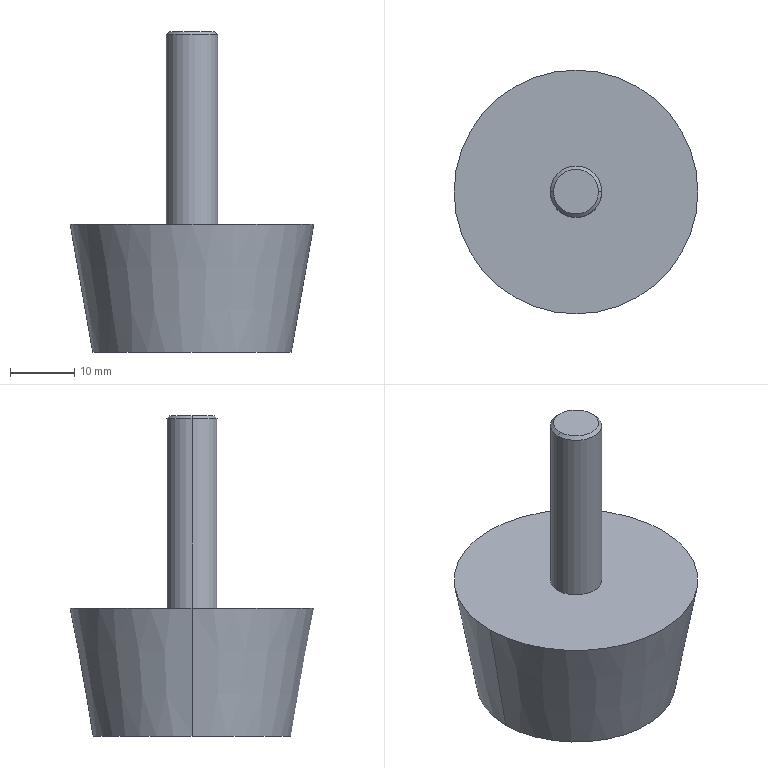Part | SolidWorks | features Chamfer 2, MoveCopyBody 2, Extrusion 1, ICE 1 | 1 solid | 9 faces | box 38 x 38 x 50 mm | volume 20238 mm3 | cone 4 | plane 3 | cylinder 2 | commonest cylinder face diameters 8 x2
STEP:
#1=CARTESIAN_POINT('',(3.5,0.,30.));
#2=VERTEX_POINT('',#1);
#3=CARTESIAN_POINT('',(-3.5,0.,30.));
#4=VERTEX_POINT('',#3);
#5=CARTESIAN_POINT('',(0.,0.,30.));
#6=DIRECTION('',(0.,0.,-1.));
#7=DIRECTION('',(-1.,0.,0.));
#8=AXIS2_PLACEMENT_3D('',#5,#6,#7);
#9=CIRCLE('',#8,3.5);
#10=EDGE_CURVE('',#2,#4,#9,.T.);
#11=ORIENTED_EDGE('',*,*,#10,.T.);
#12=CARTESIAN_POINT('',(-4.,0.,29.5));
#13=VERTEX_POINT('',#12);
#14=CARTESIAN_POINT('',(-3.5,0.,30.));
#15=DIRECTION('',(-0.7071,0.,-0.7071));
#16=VECTOR('',#15,1000.);
#17=LINE('',#14,#16);
#18=EDGE_CURVE('',#4,#13,#17,.T.);
#19=ORIENTED_EDGE('',*,*,#18,.T.);
#20=CARTESIAN_POINT('',(4.,0.,29.5));
#21=VERTEX_POINT('',#20);
#22=CARTESIAN_POINT('',(0.,0.,29.5));
#23=DIRECTION('',(0.,0.,1.));
#24=DIRECTION('',(-1.,0.,0.));
#25=AXIS2_PLACEMENT_3D('',#22,#23,#24);
#26=CIRCLE('',#25,4.);
#27=EDGE_CURVE('',#13,#21,#26,.T.);
#28=ORIENTED_EDGE('',*,*,#27,.T.);
#29=CARTESIAN_POINT('',(3.5,0.,30.));
#30=DIRECTION('',(0.7071,0.,-0.7071));
#31=VECTOR('',#30,1000.);
#32=LINE('',#29,#31);
#33=EDGE_CURVE('',#2,#21,#32,.T.);
#34=ORIENTED_EDGE('',*,*,#33,.F.);
#35=EDGE_LOOP('',(#11,#19,#28,#34));
#36=FACE_OUTER_BOUND('',#35,.T.);
#37=CARTESIAN_POINT('',(0.,0.,30.));
#38=DIRECTION('',(0.,0.,-1.));
#39=DIRECTION('',(1.,0.,0.));
#40=AXIS2_PLACEMENT_3D('',#37,#38,#39);
#41=CONICAL_SURFACE('',#40,3.5,0.7854);
#42=ADVANCED_FACE('',(#36),#41,.T.);
#43=ORIENTED_EDGE('',*,*,#27,.F.);
#44=CARTESIAN_POINT('',(-4.,0.,0.));
#45=VERTEX_POINT('',#44);
#46=CARTESIAN_POINT('',(-4.,0.,30.));
#47=DIRECTION('',(0.,0.,-1.));
#48=VECTOR('',#47,1000.);
#49=LINE('',#46,#48);
#50=EDGE_CURVE('',#13,#45,#49,.T.);
#51=ORIENTED_EDGE('',*,*,#50,.T.);
#52=CARTESIAN_POINT('',(4.,0.,0.));
#53=VERTEX_POINT('',#52);
#54=CARTESIAN_POINT('',(0.,0.,0.));
#55=DIRECTION('',(0.,0.,-1.));
#56=DIRECTION('',(-1.,0.,0.));
#57=AXIS2_PLACEMENT_3D('',#54,#55,#56);
#58=CIRCLE('',#57,4.);
#59=EDGE_CURVE('',#53,#45,#58,.T.);
#60=ORIENTED_EDGE('',*,*,#59,.F.);
#61=CARTESIAN_POINT('',(4.,0.,30.));
#62=DIRECTION('',(0.,0.,-1.));
#63=VECTOR('',#62,1000.);
#64=LINE('',#61,#63);
#65=EDGE_CURVE('',#21,#53,#64,.T.);
#66=ORIENTED_EDGE('',*,*,#65,.F.);
#67=EDGE_LOOP('',(#43,#51,#60,#66));
#68=FACE_OUTER_BOUND('',#67,.T.);
#69=CARTESIAN_POINT('',(0.,0.,30.));
#70=DIRECTION('',(0.,0.,-1.));
#71=DIRECTION('',(1.,0.,0.));
#72=AXIS2_PLACEMENT_3D('',#69,#70,#71);
#73=CYLINDRICAL_SURFACE('',#72,4.);
#74=ADVANCED_FACE('',(#68),#73,.T.);
#75=CARTESIAN_POINT('',(-15.473,0.,-20.));
#76=VERTEX_POINT('',#75);
#77=CARTESIAN_POINT('',(15.473,0.,-20.));
#78=VERTEX_POINT('',#77);
#79=CARTESIAN_POINT('',(0.,0.,-20.));
#80=DIRECTION('',(0.,0.,1.));
#81=DIRECTION('',(1.,0.,0.));
#82=AXIS2_PLACEMENT_3D('',#79,#80,#81);
#83=CIRCLE('',#82,15.473);
#84=EDGE_CURVE('',#76,#78,#83,.T.);
#85=ORIENTED_EDGE('',*,*,#84,.T.);
#86=CARTESIAN_POINT('',(19.,0.,0.));
#87=VERTEX_POINT('',#86);
#88=CARTESIAN_POINT('',(15.473,0.,-20.));
#89=DIRECTION('',(0.1736,0.,0.9848));
#90=VECTOR('',#89,1000.);
#91=LINE('',#88,#90);
#92=EDGE_CURVE('',#78,#87,#91,.T.);
#93=ORIENTED_EDGE('',*,*,#92,.T.);
#94=CARTESIAN_POINT('',(-19.,0.,0.));
#95=VERTEX_POINT('',#94);
#96=CARTESIAN_POINT('',(0.,0.,0.));
#97=DIRECTION('',(0.,0.,1.));
#98=DIRECTION('',(1.,0.,0.));
#99=AXIS2_PLACEMENT_3D('',#96,#97,#98);
#100=CIRCLE('',#99,19.);
#101=EDGE_CURVE('',#95,#87,#100,.T.);
#102=ORIENTED_EDGE('',*,*,#101,.F.);
#103=CARTESIAN_POINT('',(-15.473,0.,-20.));
#104=DIRECTION('',(-0.1736,0.,0.9848));
#105=VECTOR('',#104,1000.);
#106=LINE('',#103,#105);
#107=EDGE_CURVE('',#76,#95,#106,.T.);
#108=ORIENTED_EDGE('',*,*,#107,.F.);
#109=EDGE_LOOP('',(#85,#93,#102,#108));
#110=FACE_OUTER_BOUND('',#109,.T.);
#111=CARTESIAN_POINT('',(0.,0.,-20.));
#112=DIRECTION('',(0.,0.,1.));
#113=DIRECTION('',(-1.,0.,0.));
#114=AXIS2_PLACEMENT_3D('',#111,#112,#113);
#115=CONICAL_SURFACE('',#114,15.473,0.1745);
#116=ADVANCED_FACE('',(#110),#115,.T.);
#117=ORIENTED_EDGE('',*,*,#84,.F.);
#118=CARTESIAN_POINT('',(0.,0.,-20.));
#119=DIRECTION('',(0.,0.,1.));
#120=DIRECTION('',(1.,0.,0.));
#121=AXIS2_PLACEMENT_3D('',#118,#119,#120);
#122=CIRCLE('',#121,15.473);
#123=EDGE_CURVE('',#78,#76,#122,.T.);
#124=ORIENTED_EDGE('',*,*,#123,.F.);
#125=EDGE_LOOP('',(#117,#124));
#126=FACE_OUTER_BOUND('',#125,.T.);
#127=CARTESIAN_POINT('',(0.,0.,-20.));
#128=DIRECTION('',(0.,0.,-1.));
#129=DIRECTION('',(1.,0.,0.));
#130=AXIS2_PLACEMENT_3D('',#127,#128,#129);
#131=PLANE('',#130);
#132=ADVANCED_FACE('',(#126),#131,.T.);
#133=ORIENTED_EDGE('',*,*,#59,.T.);
#134=CARTESIAN_POINT('',(0.,0.,0.));
#135=DIRECTION('',(0.,0.,-1.));
#136=DIRECTION('',(-1.,0.,0.));
#137=AXIS2_PLACEMENT_3D('',#134,#135,#136);
#138=CIRCLE('',#137,4.);
#139=EDGE_CURVE('',#45,#53,#138,.T.);
#140=ORIENTED_EDGE('',*,*,#139,.T.);
#141=EDGE_LOOP('',(#133,#140));
#142=FACE_BOUND('',#141,.T.);
#143=ORIENTED_EDGE('',*,*,#101,.T.);
#144=CARTESIAN_POINT('',(0.,0.,0.));
#145=DIRECTION('',(0.,0.,1.));
#146=DIRECTION('',(1.,0.,0.));
#147=AXIS2_PLACEMENT_3D('',#144,#145,#146);
#148=CIRCLE('',#147,19.);
#149=EDGE_CURVE('',#87,#95,#148,.T.);
#150=ORIENTED_EDGE('',*,*,#149,.T.);
#151=EDGE_LOOP('',(#143,#150));
#152=FACE_OUTER_BOUND('',#151,.T.);
#153=CARTESIAN_POINT('',(0.,0.,0.));
#154=DIRECTION('',(0.,0.,-1.));
#155=DIRECTION('',(1.,0.,0.));
#156=AXIS2_PLACEMENT_3D('',#153,#154,#155);
#157=PLANE('',#156);
#158=ADVANCED_FACE('',(#142,#152),#157,.F.);
#159=ORIENTED_EDGE('',*,*,#92,.F.);
#160=ORIENTED_EDGE('',*,*,#123,.T.);
#161=ORIENTED_EDGE('',*,*,#107,.T.);
#162=ORIENTED_EDGE('',*,*,#149,.F.);
#163=EDGE_LOOP('',(#159,#160,#161,#162));
#164=FACE_OUTER_BOUND('',#163,.T.);
#165=CARTESIAN_POINT('',(0.,0.,-20.));
#166=DIRECTION('',(0.,0.,1.));
#167=DIRECTION('',(-1.,0.,0.));
#168=AXIS2_PLACEMENT_3D('',#165,#166,#167);
#169=CONICAL_SURFACE('',#168,15.473,0.1745);
#170=ADVANCED_FACE('',(#164),#169,.T.);
#171=ORIENTED_EDGE('',*,*,#50,.F.);
#172=CARTESIAN_POINT('',(0.,0.,29.5));
#173=DIRECTION('',(0.,0.,1.));
#174=DIRECTION('',(-1.,0.,0.));
#175=AXIS2_PLACEMENT_3D('',#172,#173,#174);
#176=CIRCLE('',#175,4.);
#177=EDGE_CURVE('',#21,#13,#176,.T.);
#178=ORIENTED_EDGE('',*,*,#177,.F.);
#179=ORIENTED_EDGE('',*,*,#65,.T.);
#180=ORIENTED_EDGE('',*,*,#139,.F.);
#181=EDGE_LOOP('',(#171,#178,#179,#180));
#182=FACE_OUTER_BOUND('',#181,.T.);
#183=CARTESIAN_POINT('',(0.,0.,30.));
#184=DIRECTION('',(0.,0.,-1.));
#185=DIRECTION('',(1.,0.,0.));
#186=AXIS2_PLACEMENT_3D('',#183,#184,#185);
#187=CYLINDRICAL_SURFACE('',#186,4.);
#188=ADVANCED_FACE('',(#182),#187,.T.);
#189=ORIENTED_EDGE('',*,*,#10,.F.);
#190=CARTESIAN_POINT('',(0.,0.,30.));
#191=DIRECTION('',(0.,0.,-1.));
#192=DIRECTION('',(-1.,0.,0.));
#193=AXIS2_PLACEMENT_3D('',#190,#191,#192);
#194=CIRCLE('',#193,3.5);
#195=EDGE_CURVE('',#4,#2,#194,.T.);
#196=ORIENTED_EDGE('',*,*,#195,.F.);
#197=EDGE_LOOP('',(#189,#196));
#198=FACE_OUTER_BOUND('',#197,.T.);
#199=CARTESIAN_POINT('',(0.,0.,30.));
#200=DIRECTION('',(0.,0.,1.));
#201=DIRECTION('',(-1.,0.,0.));
#202=AXIS2_PLACEMENT_3D('',#199,#200,#201);
#203=PLANE('',#202);
#204=ADVANCED_FACE('',(#198),#203,.T.);
#205=ORIENTED_EDGE('',*,*,#18,.F.);
#206=ORIENTED_EDGE('',*,*,#195,.T.);
#207=ORIENTED_EDGE('',*,*,#33,.T.);
#208=ORIENTED_EDGE('',*,*,#177,.T.);
#209=EDGE_LOOP('',(#205,#206,#207,#208));
#210=FACE_OUTER_BOUND('',#209,.T.);
#211=CARTESIAN_POINT('',(0.,0.,30.));
#212=DIRECTION('',(0.,0.,-1.));
#213=DIRECTION('',(1.,0.,0.));
#214=AXIS2_PLACEMENT_3D('',#211,#212,#213);
#215=CONICAL_SURFACE('',#214,3.5,0.7854);
#216=ADVANCED_FACE('',(#210),#215,.T.);
#217=CLOSED_SHELL('',(#42,#74,#116,#132,#158,#170,#188,#204,#216));
#218=MANIFOLD_SOLID_BREP('',#217);
#219=CARTESIAN_POINT('',(0.,0.,0.));
#220=DIRECTION('',(0.,0.,1.));
#221=DIRECTION('',(1.,0.,0.));
#222=AXIS2_PLACEMENT_3D('',#219,#220,#221);
#223=(LENGTH_UNIT()NAMED_UNIT(*)SI_UNIT(.MILLI.,.METRE.));
#224=UNCERTAINTY_MEASURE_WITH_UNIT(LENGTH_MEASURE(0.00001),#223,'','');
#225=(NAMED_UNIT(*)PLANE_ANGLE_UNIT()SI_UNIT($,.RADIAN.));
#226=(NAMED_UNIT(*)SI_UNIT($,.STERADIAN.)SOLID_ANGLE_UNIT());
#227=(GEOMETRIC_REPRESENTATION_CONTEXT(3)GLOBAL_UNCERTAINTY_ASSIGNED_CONTEXT((#224))GLOBAL_UNIT_ASSIGNED_CONTEXT((#223,#225,#226))REPRESENTATION_CONTEXT('',''));
#228=ADVANCED_BREP_SHAPE_REPRESENTATION('',(#218,#222),#227);